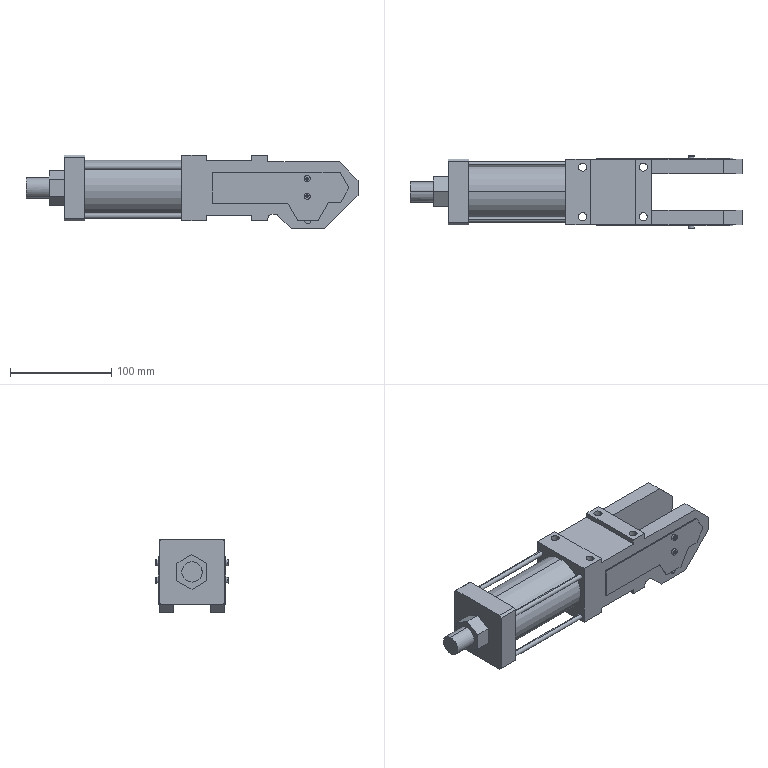Part | STEP file | Positioning_id1918_x_t | 1 solid | 168 faces | box 328 x 72 x 73 mm | volume 808881 mm3 | plane 128 | cylinder 36 | torus 4 | commonest cylinder face diameters 6 x12 8 x12 5 x8 20 x2 55 x2